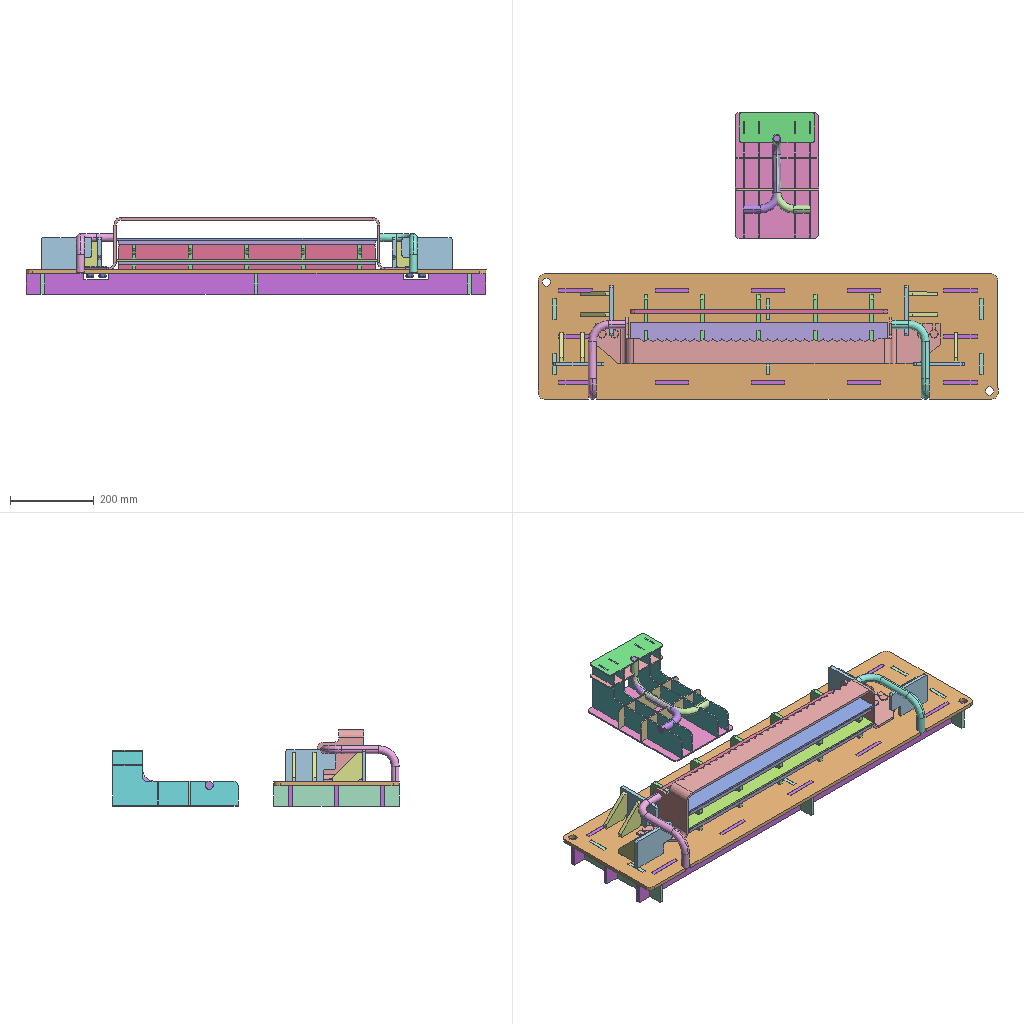Assembly | SolidWorks | 20 different items | 48 placed | box 1100 x 685 x 184 mm
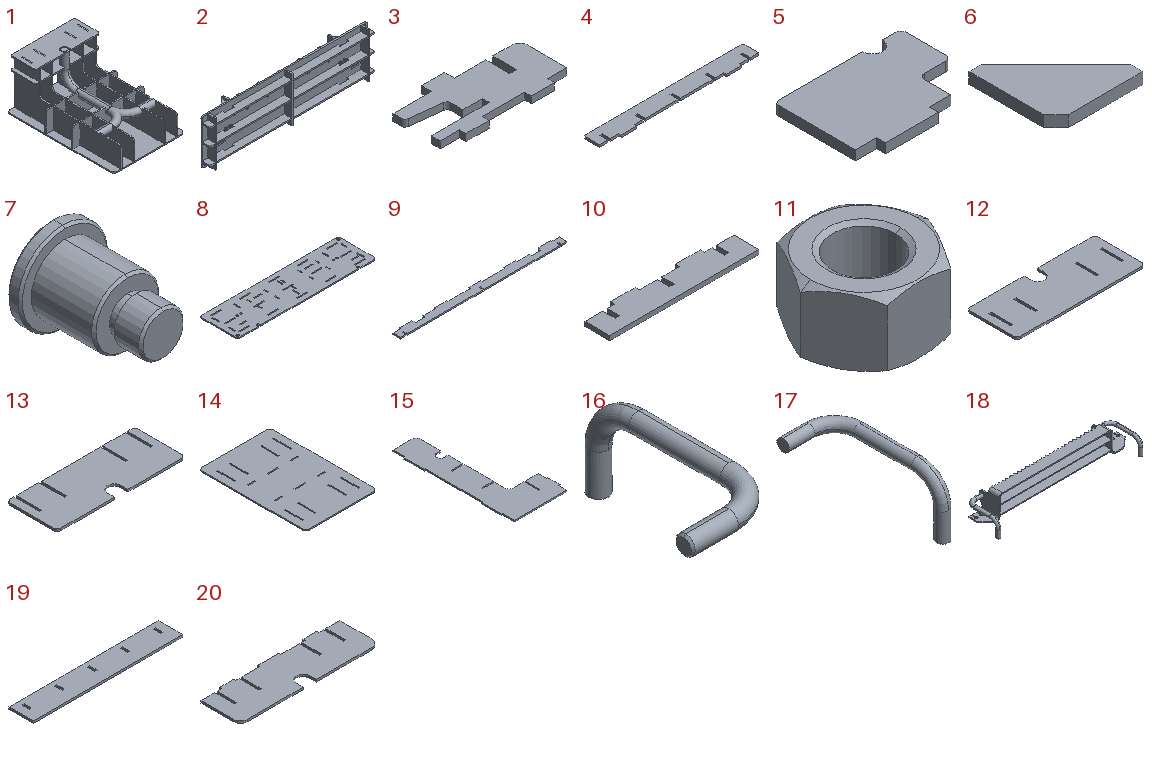Parts list (item | name | quantity | parent item | size | volume | features):
1 | (subassembly) | x1 | - | 200 x 300 x 135 mm | 782542 mm3 | features ReferencePattern 4, LocalLPattern 3, MirrorCompFeat 1
2 | (subassembly) | x1 | - | 1100 x 184 x 300 mm | 7919569 mm3 | features ReferencePattern 16, LocalLPattern 6, MirrorCompFeat 1
3 | - | x5 | in 2 | 165 x 83 x 9 mm | 80282 mm3 | features FlatPattern 1, SMBaseFlange 1, SheetMetal 1
4 | - | x1 | in 2 | 615 x 70 x 9 mm | 336641 mm3 | features FlatPattern 1, SMBaseFlange 1, SheetMetal 1
5 | - | x4 | in 2 | 120 x 85.5 x 9 mm | 77513 mm3 | features FlatPattern 1, SMBaseFlange 1, SheetMetal 1
6 | - | x7 | in 2 | 70 x 70 x 9 mm | 27450 mm3 | features FlatPattern 1, SMBaseFlange 1, SheetMetal 1
7 | - | x4 | in 2 | 20 x 25 x 20 mm | 3963 mm3 | features Chamfer 1, Revolution 1
8 | - | x1 | in 2 | 1100 x 300 x 9 mm | 2778509 mm3 | features FlatPattern 1, SMBaseFlange 1, SheetMetal 1
9 | - | x3 | in 2 | 1100 x 58.5 x 9 mm | 503273 mm3 | features FlatPattern 1, SMBaseFlange 1, SheetMetal 1
10 | - | x3 | in 2 | 300 x 58.5 x 9 mm | 136575 mm3 | features FlatPattern 1, SMBaseFlange 1, SheetMetal 1
11 | - | x4 | in 2 | 27.713 x 24 x 14.8 mm | 5071 mm3 | features RevCut 2, Chamfer 1, Extrusion 1, LPattern 1
12 | - | x1 | in 1 | 180 x 71 x 3.2 mm | 38567 mm3 | features FlatPattern 1, SMBaseFlange 1, SheetMetal 1
13 | - | x1 | in 1 | 180 x 71 x 3.2 mm | 38342 mm3 | features FlatPattern 1, SMBaseFlange 1, SheetMetal 1
14 | - | x1 | in 1 | 200 x 300 x 3.2 mm | 186196 mm3 | features FlatPattern 1, SMBaseFlange 1, SheetMetal 1
15 | - | x4 | in 1 | 134.6 x 300 x 3.2 mm | 70099 mm3 | features FlatPattern 1, SMBaseFlange 1, SheetMetal 1
16 | - | x1 | in 1 | 94 x 188 x 89.5 mm | 84832 mm3 | features 3DProfileFeature 2, Chamfer 1, Sweep 1
17 | - | x1 | in 1 | 89.5 x 188 x 94 mm | 84832 mm3 | features 3DProfileFeature 2, Chamfer 1, Sweep 1
18 | - | x1 | in 2 | 841.5 x 196.5 x 132.5 mm | 877492 mm3 | features BaseBody 5
19 | - | x2 | in 2 | 615 x 100 x 9 mm | 541350 mm3 | features FlatPattern 1, SMBaseFlange 1, SheetMetal 1
20 | - | x2 | in 1 | 200 x 59.8 x 3.2 mm | 34688 mm3 | features FlatPattern 1, SMBaseFlange 1, SheetMetal 1
Mates (type | each side: item.copy, entity, surface, feature):
In the top assembly
Coincident | 9.1 face plane Base-Flange1 | 14.1 face plane Base-Flange1
In subassembly 2
InPlace | 18.1 face plane 2A7-54-K1360-01-1-solid1 | 8.1 plane
InPlace | 18.1 face plane 2A7-54-K1360-02-1-solid1 | 19.1 plane
InPlace | 3.1 plane | 2.1 plane
InPlace | 4.1 plane | 2.1 plane
InPlace | 5.1 plane | 2.1 plane
Concentric | 18.1 face cylinder 2A7-54-K1360-03-1-solid1 | 5.2 face cylinder Base-Flange1
DistanceDim | 18.1 face plane 2A7-54-K1360-01-1-solid1 | 5.2 face plane Base-Flange1
InPlace | 6.1 plane | 2.1 plane
Coincident | 5.1 face plane Base-Flange1 | 6.2 face plane Base-Flange1
Coincident | 8.1 face plane Base-Flange1 | 6.2 face plane Base-Flange1
DistanceDim | 5.1 face plane Base-Flange1 | 6.2 face plane Base-Flange1
InPlace | 9.2 plane | 2.1 plane
InPlace | 10.1 plane | 2.1 plane
Concentric | 18.1 face cylinder 2A7-54-K1360-01-1-solid1 | 7.1 face cylinder Revolve1
Coincident | 18.1 face plane 2A7-54-K1360-01-1-solid1 | 7.1 face plane Revolve1
Concentric | 18.1 face cylinder 2A7-54-K1360-01-1-solid1 | 7.2 face cylinder Revolve1
Coincident | 7.1 face plane Revolve1 | 7.2 face plane Revolve1
Concentric | 18.1 face cylinder 2A7-54-K1360-01-1-solid1 | 7.3 face cylinder Revolve1
Coincident | 18.1 face plane 2A7-54-K1360-01-1-solid1 | 7.3 face plane Revolve1
Concentric | 18.1 face cylinder 2A7-54-K1360-01-1-solid1 | 7.4 face cylinder Revolve1
Coincident | 7.3 face plane Revolve1 | 7.4 face plane Revolve1
Concentric | 8.1 face cylinder Base-Flange1 | 11.1 face cone EndChamfer
Coincident | 8.1 face plane Base-Flange1 | 11.1 face plane BaseNut
Concentric | 8.1 face cylinder Base-Flange1 | 11.2 face cone EndChamfer
Coincident | 8.1 face plane Base-Flange1 | 11.2 face plane BaseNut
Concentric | 8.1 face cylinder Base-Flange1 | 11.3 face cone EndChamfer
Coincident | 8.1 face plane Base-Flange1 | 11.3 face plane BaseNut
Concentric | 8.1 face cylinder Base-Flange1 | 11.4 face cone EndChamfer
Coincident | 8.1 face plane Base-Flange1 | 11.4 face plane BaseNut
In subassembly 1
InPlace | 14.2 plane | 1.1 plane
InPlace | 16.1 face plane Sweep1 | 15.1 plane
InPlace | 20.1 plane | 1.1 plane
Concentric | 16.1 face cylinder Sweep1 | 17.1 face cylinder Sweep1 | 2 times
Coincident | 16.1 face plane Sweep1 | 17.1 face plane Sweep1
InPlace | 15.2 face plane Base-Flange1 | 12.1 plane
InPlace | 13.1 plane | 1.1 plane